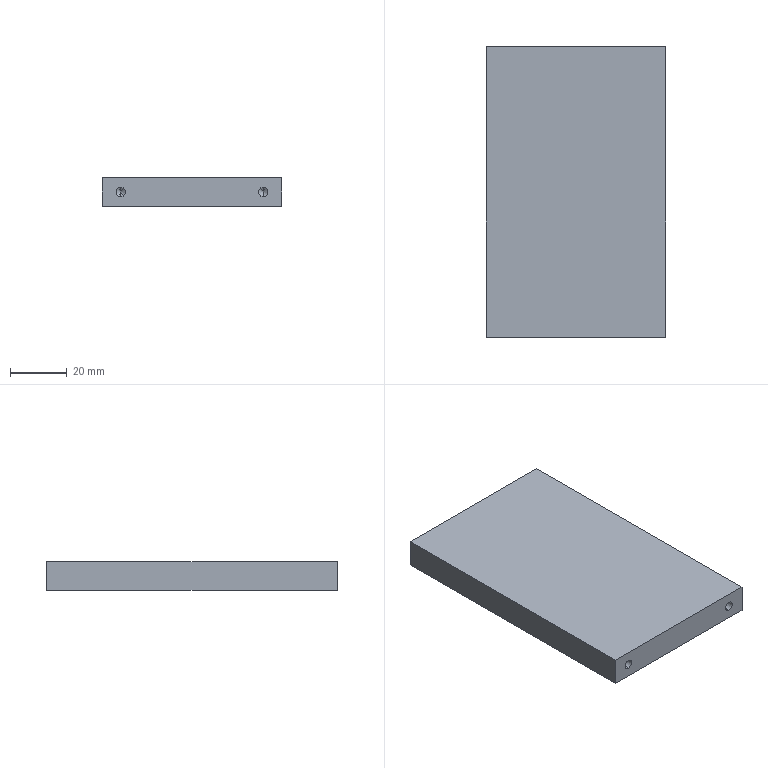Part | STEP file | 2033 Reinforcing rib | 1 solid | 22 faces | box 63 x 102 x 10 mm | volume 63855 mm3 | cylinder 8 | cone 8 | plane 6 | commonest cylinder face diameters 3.3 x8
STEP:
#1=CARTESIAN_POINT('',(0.,0.,0.));
#2=DIRECTION('',(0.,0.,1.));
#3=DIRECTION('',(1.,0.,0.));
#4=AXIS2_PLACEMENT_3D('',#1,#2,#3);
#5=CARTESIAN_POINT('',(56.5,90.5,6.65));
#6=VERTEX_POINT('',#5);
#7=CARTESIAN_POINT('',(56.5,102.,6.65));
#8=VERTEX_POINT('',#7);
#9=CARTESIAN_POINT('',(56.5,102.,6.65));
#10=DIRECTION('',(0.,1.,0.));
#11=VECTOR('',#10,1.);
#12=LINE('',#9,#11);
#13=CARTESIAN_POINT('',(56.5,102.,5.));
#14=DIRECTION('',(0.,1.,0.));
#15=DIRECTION('',(0.,0.,1.));
#16=AXIS2_PLACEMENT_3D('',#13,#14,#15);
#17=CYLINDRICAL_SURFACE('',#16,1.65);
#18=CARTESIAN_POINT('',(6.283,0.));
#19=DIRECTION('',(0.,1.));
#20=VECTOR('',#19,1.);
#21=LINE('',#18,#20);
#22=(GEOMETRIC_REPRESENTATION_CONTEXT(2)PARAMETRIC_REPRESENTATION_CONTEXT()REPRESENTATION_CONTEXT('',''));
#23=DEFINITIONAL_REPRESENTATION('',(#21),#22);
#24=PCURVE('',#17,#23);
#25=CARTESIAN_POINT('',(56.5,102.,5.));
#26=DIRECTION('',(0.,1.,0.));
#27=DIRECTION('',(0.,0.,1.));
#28=AXIS2_PLACEMENT_3D('',#25,#26,#27);
#29=CYLINDRICAL_SURFACE('',#28,1.65);
#30=CARTESIAN_POINT('',(0.,0.));
#31=DIRECTION('',(0.,1.));
#32=VECTOR('',#31,1.);
#33=LINE('',#30,#32);
#34=(GEOMETRIC_REPRESENTATION_CONTEXT(2)PARAMETRIC_REPRESENTATION_CONTEXT()REPRESENTATION_CONTEXT('',''));
#35=DEFINITIONAL_REPRESENTATION('',(#33),#34);
#36=PCURVE('',#29,#35);
#37=SURFACE_CURVE('',#12,(#24,#36),.PCURVE_S1.);
#38=EDGE_CURVE('',#6,#8,#37,.T.);
#39=ORIENTED_EDGE('',*,*,#38,.T.);
#40=CARTESIAN_POINT('',(56.5,102.,3.35));
#41=VERTEX_POINT('',#40);
#42=CARTESIAN_POINT('',(56.5,102.,5.));
#43=DIRECTION('',(0.,1.,0.));
#44=DIRECTION('',(0.,0.,1.));
#45=AXIS2_PLACEMENT_3D('',#42,#43,#44);
#46=CIRCLE('',#45,1.65);
#47=CARTESIAN_POINT('',(0.,0.));
#48=DIRECTION('',(1.,0.));
#49=VECTOR('',#48,1.);
#50=LINE('',#47,#49);
#51=(GEOMETRIC_REPRESENTATION_CONTEXT(2)PARAMETRIC_REPRESENTATION_CONTEXT()REPRESENTATION_CONTEXT('',''));
#52=DEFINITIONAL_REPRESENTATION('',(#50),#51);
#53=PCURVE('',#17,#52);
#54=CARTESIAN_POINT('',(63.,102.,10.));
#55=DIRECTION('',(0.,-1.,0.));
#56=DIRECTION('',(1.,0.,0.));
#57=AXIS2_PLACEMENT_3D('',#54,#55,#56);
#58=PLANE('',#57);
#59=CARTESIAN_POINT('',(-6.5,-3.35));
#60=CARTESIAN_POINT('',(-3.642,-3.35));
#61=CARTESIAN_POINT('',(-5.071,-5.825));
#62=CARTESIAN_POINT('',(-6.5,-8.3));
#63=CARTESIAN_POINT('',(-7.929,-5.825));
#64=CARTESIAN_POINT('',(-9.358,-3.35));
#65=CARTESIAN_POINT('',(-6.5,-3.35));
#66=(BOUNDED_CURVE()B_SPLINE_CURVE(2,(#59,#60,#61,#62,#63,#64,#65),.UNSPECIFIED.,.T.,.F.)B_SPLINE_CURVE_WITH_KNOTS((1,2,2,2,2,1),(-2.094,0.,2.094,4.189,6.283,8.378),.UNSPECIFIED.)CURVE()GEOMETRIC_REPRESENTATION_ITEM()RATIONAL_B_SPLINE_CURVE((1.,0.5,1.,0.5,1.,0.5,1.))REPRESENTATION_ITEM(''));
#67=(GEOMETRIC_REPRESENTATION_CONTEXT(2)PARAMETRIC_REPRESENTATION_CONTEXT()REPRESENTATION_CONTEXT('',''));
#68=DEFINITIONAL_REPRESENTATION('',(#66),#67);
#69=PCURVE('',#58,#68);
#70=SURFACE_CURVE('',#46,(#53,#69),.PCURVE_S1.);
#71=EDGE_CURVE('',#41,#8,#70,.T.);
#72=ORIENTED_EDGE('',*,*,#71,.F.);
#73=CARTESIAN_POINT('',(56.5,90.5,3.35));
#74=VERTEX_POINT('',#73);
#75=CARTESIAN_POINT('',(56.5,102.,3.35));
#76=DIRECTION('',(0.,1.,0.));
#77=VECTOR('',#76,1.);
#78=LINE('',#75,#77);
#79=CARTESIAN_POINT('',(3.142,0.));
#80=DIRECTION('',(0.,1.));
#81=VECTOR('',#80,1.);
#82=LINE('',#79,#81);
#83=(GEOMETRIC_REPRESENTATION_CONTEXT(2)PARAMETRIC_REPRESENTATION_CONTEXT()REPRESENTATION_CONTEXT('',''));
#84=DEFINITIONAL_REPRESENTATION('',(#82),#83);
#85=PCURVE('',#17,#84);
#86=CARTESIAN_POINT('',(3.142,0.));
#87=DIRECTION('',(0.,1.));
#88=VECTOR('',#87,1.);
#89=LINE('',#86,#88);
#90=(GEOMETRIC_REPRESENTATION_CONTEXT(2)PARAMETRIC_REPRESENTATION_CONTEXT()REPRESENTATION_CONTEXT('',''));
#91=DEFINITIONAL_REPRESENTATION('',(#89),#90);
#92=PCURVE('',#29,#91);
#93=SURFACE_CURVE('',#78,(#85,#92),.PCURVE_S1.);
#94=EDGE_CURVE('',#74,#41,#93,.T.);
#95=ORIENTED_EDGE('',*,*,#94,.F.);
#96=CARTESIAN_POINT('',(56.5,90.5,5.));
#97=DIRECTION('',(0.,1.,0.));
#98=DIRECTION('',(0.,0.,1.));
#99=AXIS2_PLACEMENT_3D('',#96,#97,#98);
#100=CIRCLE('',#99,1.65);
#101=CARTESIAN_POINT('',(0.,-11.5));
#102=DIRECTION('',(1.,0.));
#103=VECTOR('',#102,1.);
#104=LINE('',#101,#103);
#105=(GEOMETRIC_REPRESENTATION_CONTEXT(2)PARAMETRIC_REPRESENTATION_CONTEXT()REPRESENTATION_CONTEXT('',''));
#106=DEFINITIONAL_REPRESENTATION('',(#104),#105);
#107=PCURVE('',#17,#106);
#108=CARTESIAN_POINT('',(56.5,90.5,5.));
#109=DIRECTION('',(0.,1.,0.));
#110=DIRECTION('',(0.,0.,1.));
#111=AXIS2_PLACEMENT_3D('',#108,#109,#110);
#112=CONICAL_SURFACE('',#111,1.65,1.03);
#113=CARTESIAN_POINT('',(0.,0.));
#114=DIRECTION('',(1.,0.));
#115=VECTOR('',#114,1.);
#116=LINE('',#113,#115);
#117=(GEOMETRIC_REPRESENTATION_CONTEXT(2)PARAMETRIC_REPRESENTATION_CONTEXT()REPRESENTATION_CONTEXT('',''));
#118=DEFINITIONAL_REPRESENTATION('',(#116),#117);
#119=PCURVE('',#112,#118);
#120=SURFACE_CURVE('',#100,(#107,#119),.PCURVE_S1.);
#121=EDGE_CURVE('',#74,#6,#120,.T.);
#122=ORIENTED_EDGE('',*,*,#121,.T.);
#123=EDGE_LOOP('',(#39,#72,#95,#122));
#124=FACE_BOUND('',#123,.F.);
#125=ADVANCED_FACE('',(#124),#17,.F.);
#126=ORIENTED_EDGE('',*,*,#121,.F.);
#127=CARTESIAN_POINT('',(56.5,89.509,5.));
#128=VERTEX_POINT('',#127);
#129=CARTESIAN_POINT('',(56.5,90.5,3.35));
#130=DIRECTION('',(0.,0.515,-0.8572));
#131=VECTOR('',#130,1.);
#132=LINE('',#129,#131);
#133=CARTESIAN_POINT('',(3.142,0.));
#134=DIRECTION('',(0.,1.));
#135=VECTOR('',#134,1.);
#136=LINE('',#133,#135);
#137=(GEOMETRIC_REPRESENTATION_CONTEXT(2)PARAMETRIC_REPRESENTATION_CONTEXT()REPRESENTATION_CONTEXT('',''));
#138=DEFINITIONAL_REPRESENTATION('',(#136),#137);
#139=PCURVE('',#112,#138);
#140=CARTESIAN_POINT('',(56.5,90.5,5.));
#141=DIRECTION('',(0.,1.,0.));
#142=DIRECTION('',(0.,0.,1.));
#143=AXIS2_PLACEMENT_3D('',#140,#141,#142);
#144=CONICAL_SURFACE('',#143,1.65,1.03);
#145=CARTESIAN_POINT('',(3.142,0.));
#146=DIRECTION('',(0.,1.));
#147=VECTOR('',#146,1.);
#148=LINE('',#145,#147);
#149=(GEOMETRIC_REPRESENTATION_CONTEXT(2)PARAMETRIC_REPRESENTATION_CONTEXT()REPRESENTATION_CONTEXT('',''));
#150=DEFINITIONAL_REPRESENTATION('',(#148),#149);
#151=PCURVE('',#144,#150);
#152=SURFACE_CURVE('',#132,(#139,#151),.PCURVE_S1.);
#153=EDGE_CURVE('',#128,#74,#152,.T.);
#154=ORIENTED_EDGE('',*,*,#153,.F.);
#155=CARTESIAN_POINT('',(56.5,90.5,6.65));
#156=DIRECTION('',(0.,0.515,0.8572));
#157=VECTOR('',#156,1.);
#158=LINE('',#155,#157);
#159=CARTESIAN_POINT('',(6.283,0.));
#160=DIRECTION('',(0.,1.));
#161=VECTOR('',#160,1.);
#162=LINE('',#159,#161);
#163=(GEOMETRIC_REPRESENTATION_CONTEXT(2)PARAMETRIC_REPRESENTATION_CONTEXT()REPRESENTATION_CONTEXT('',''));
#164=DEFINITIONAL_REPRESENTATION('',(#162),#163);
#165=PCURVE('',#112,#164);
#166=CARTESIAN_POINT('',(0.,0.));
#167=DIRECTION('',(0.,1.));
#168=VECTOR('',#167,1.);
#169=LINE('',#166,#168);
#170=(GEOMETRIC_REPRESENTATION_CONTEXT(2)PARAMETRIC_REPRESENTATION_CONTEXT()REPRESENTATION_CONTEXT('',''));
#171=DEFINITIONAL_REPRESENTATION('',(#169),#170);
#172=PCURVE('',#144,#171);
#173=SURFACE_CURVE('',#158,(#165,#172),.PCURVE_S1.);
#174=EDGE_CURVE('',#128,#6,#173,.T.);
#175=ORIENTED_EDGE('',*,*,#174,.T.);
#176=EDGE_LOOP('',(#126,#154,#175));
#177=FACE_BOUND('',#176,.F.);
#178=ADVANCED_FACE('',(#177),#112,.F.);
#179=CARTESIAN_POINT('',(6.5,90.5,6.65));
#180=VERTEX_POINT('',#179);
#181=CARTESIAN_POINT('',(6.5,102.,6.65));
#182=VERTEX_POINT('',#181);
#183=CARTESIAN_POINT('',(6.5,102.,6.65));
#184=DIRECTION('',(0.,1.,0.));
#185=VECTOR('',#184,1.);
#186=LINE('',#183,#185);
#187=CARTESIAN_POINT('',(6.5,102.,5.));
#188=DIRECTION('',(0.,1.,0.));
#189=DIRECTION('',(0.,0.,1.));
#190=AXIS2_PLACEMENT_3D('',#187,#188,#189);
#191=CYLINDRICAL_SURFACE('',#190,1.65);
#192=CARTESIAN_POINT('',(6.283,0.));
#193=DIRECTION('',(0.,1.));
#194=VECTOR('',#193,1.);
#195=LINE('',#192,#194);
#196=(GEOMETRIC_REPRESENTATION_CONTEXT(2)PARAMETRIC_REPRESENTATION_CONTEXT()REPRESENTATION_CONTEXT('',''));
#197=DEFINITIONAL_REPRESENTATION('',(#195),#196);
#198=PCURVE('',#191,#197);
#199=CARTESIAN_POINT('',(6.5,102.,5.));
#200=DIRECTION('',(0.,1.,0.));
#201=DIRECTION('',(0.,0.,1.));
#202=AXIS2_PLACEMENT_3D('',#199,#200,#201);
#203=CYLINDRICAL_SURFACE('',#202,1.65);
#204=CARTESIAN_POINT('',(0.,0.));
#205=DIRECTION('',(0.,1.));
#206=VECTOR('',#205,1.);
#207=LINE('',#204,#206);
#208=(GEOMETRIC_REPRESENTATION_CONTEXT(2)PARAMETRIC_REPRESENTATION_CONTEXT()REPRESENTATION_CONTEXT('',''));
#209=DEFINITIONAL_REPRESENTATION('',(#207),#208);
#210=PCURVE('',#203,#209);
#211=SURFACE_CURVE('',#186,(#198,#210),.PCURVE_S1.);
#212=EDGE_CURVE('',#180,#182,#211,.T.);
#213=ORIENTED_EDGE('',*,*,#212,.T.);
#214=CARTESIAN_POINT('',(6.5,102.,3.35));
#215=VERTEX_POINT('',#214);
#216=CARTESIAN_POINT('',(6.5,102.,5.));
#217=DIRECTION('',(0.,1.,0.));
#218=DIRECTION('',(0.,0.,1.));
#219=AXIS2_PLACEMENT_3D('',#216,#217,#218);
#220=CIRCLE('',#219,1.65);
#221=CARTESIAN_POINT('',(0.,0.));
#222=DIRECTION('',(1.,0.));
#223=VECTOR('',#222,1.);
#224=LINE('',#221,#223);
#225=(GEOMETRIC_REPRESENTATION_CONTEXT(2)PARAMETRIC_REPRESENTATION_CONTEXT()REPRESENTATION_CONTEXT('',''));
#226=DEFINITIONAL_REPRESENTATION('',(#224),#225);
#227=PCURVE('',#191,#226);
#228=CARTESIAN_POINT('',(-56.5,-3.35));
#229=CARTESIAN_POINT('',(-53.642,-3.35));
#230=CARTESIAN_POINT('',(-55.071,-5.825));
#231=CARTESIAN_POINT('',(-56.5,-8.3));
#232=CARTESIAN_POINT('',(-57.929,-5.825));
#233=CARTESIAN_POINT('',(-59.358,-3.35));
#234=CARTESIAN_POINT('',(-56.5,-3.35));
#235=(BOUNDED_CURVE()B_SPLINE_CURVE(2,(#228,#229,#230,#231,#232,#233,#234),.UNSPECIFIED.,.T.,.F.)B_SPLINE_CURVE_WITH_KNOTS((1,2,2,2,2,1),(-2.094,0.,2.094,4.189,6.283,8.378),.UNSPECIFIED.)CURVE()GEOMETRIC_REPRESENTATION_ITEM()RATIONAL_B_SPLINE_CURVE((1.,0.5,1.,0.5,1.,0.5,1.))REPRESENTATION_ITEM(''));
#236=(GEOMETRIC_REPRESENTATION_CONTEXT(2)PARAMETRIC_REPRESENTATION_CONTEXT()REPRESENTATION_CONTEXT('',''));
#237=DEFINITIONAL_REPRESENTATION('',(#235),#236);
#238=PCURVE('',#58,#237);
#239=SURFACE_CURVE('',#220,(#227,#238),.PCURVE_S1.);
#240=EDGE_CURVE('',#215,#182,#239,.T.);
#241=ORIENTED_EDGE('',*,*,#240,.F.);
#242=CARTESIAN_POINT('',(6.5,90.5,3.35));
#243=VERTEX_POINT('',#242);
#244=CARTESIAN_POINT('',(6.5,102.,3.35));
#245=DIRECTION('',(0.,1.,0.));
#246=VECTOR('',#245,1.);
#247=LINE('',#244,#246);
#248=CARTESIAN_POINT('',(3.142,0.));
#249=DIRECTION('',(0.,1.));
#250=VECTOR('',#249,1.);
#251=LINE('',#248,#250);
#252=(GEOMETRIC_REPRESENTATION_CONTEXT(2)PARAMETRIC_REPRESENTATION_CONTEXT()REPRESENTATION_CONTEXT('',''));
#253=DEFINITIONAL_REPRESENTATION('',(#251),#252);
#254=PCURVE('',#191,#253);
#255=CARTESIAN_POINT('',(3.142,0.));
#256=DIRECTION('',(0.,1.));
#257=VECTOR('',#256,1.);
#258=LINE('',#255,#257);
#259=(GEOMETRIC_REPRESENTATION_CONTEXT(2)PARAMETRIC_REPRESENTATION_CONTEXT()REPRESENTATION_CONTEXT('',''));
#260=DEFINITIONAL_REPRESENTATION('',(#258),#259);
#261=PCURVE('',#203,#260);
#262=SURFACE_CURVE('',#247,(#254,#261),.PCURVE_S1.);
#263=EDGE_CURVE('',#243,#215,#262,.T.);
#264=ORIENTED_EDGE('',*,*,#263,.F.);
#265=CARTESIAN_POINT('',(6.5,90.5,5.));
#266=DIRECTION('',(0.,1.,0.));
#267=DIRECTION('',(0.,0.,1.));
#268=AXIS2_PLACEMENT_3D('',#265,#266,#267);
#269=CIRCLE('',#268,1.65);
#270=CARTESIAN_POINT('',(0.,-11.5));
#271=DIRECTION('',(1.,0.));
#272=VECTOR('',#271,1.);
#273=LINE('',#270,#272);
#274=(GEOMETRIC_REPRESENTATION_CONTEXT(2)PARAMETRIC_REPRESENTATION_CONTEXT()REPRESENTATION_CONTEXT('',''));
#275=DEFINITIONAL_REPRESENTATION('',(#273),#274);
#276=PCURVE('',#191,#275);
#277=CARTESIAN_POINT('',(6.5,90.5,5.));
#278=DIRECTION('',(0.,1.,0.));
#279=DIRECTION('',(0.,0.,1.));
#280=AXIS2_PLACEMENT_3D('',#277,#278,#279);
#281=CONICAL_SURFACE('',#280,1.65,1.03);
#282=CARTESIAN_POINT('',(0.,0.));
#283=DIRECTION('',(1.,0.));
#284=VECTOR('',#283,1.);
#285=LINE('',#282,#284);
#286=(GEOMETRIC_REPRESENTATION_CONTEXT(2)PARAMETRIC_REPRESENTATION_CONTEXT()REPRESENTATION_CONTEXT('',''));
#287=DEFINITIONAL_REPRESENTATION('',(#285),#286);
#288=PCURVE('',#281,#287);
#289=SURFACE_CURVE('',#269,(#276,#288),.PCURVE_S1.);
#290=EDGE_CURVE('',#243,#180,#289,.T.);
#291=ORIENTED_EDGE('',*,*,#290,.T.);
#292=EDGE_LOOP('',(#213,#241,#264,#291));
#293=FACE_BOUND('',#292,.F.);
#294=ADVANCED_FACE('',(#293),#191,.F.);
#295=ORIENTED_EDGE('',*,*,#290,.F.);
#296=CARTESIAN_POINT('',(6.5,89.509,5.));
#297=VERTEX_POINT('',#296);
#298=CARTESIAN_POINT('',(6.5,90.5,3.35));
#299=DIRECTION('',(0.,0.515,-0.8572));
#300=VECTOR('',#299,1.);
#301=LINE('',#298,#300);
#302=CARTESIAN_POINT('',(3.142,0.));
#303=DIRECTION('',(0.,1.));
#304=VECTOR('',#303,1.);
#305=LINE('',#302,#304);
#306=(GEOMETRIC_REPRESENTATION_CONTEXT(2)PARAMETRIC_REPRESENTATION_CONTEXT()REPRESENTATION_CONTEXT('',''));
#307=DEFINITIONAL_REPRESENTATION('',(#305),#306);
#308=PCURVE('',#281,#307);
#309=CARTESIAN_POINT('',(6.5,90.5,5.));
#310=DIRECTION('',(0.,1.,0.));
#311=DIRECTION('',(0.,0.,1.));
#312=AXIS2_PLACEMENT_3D('',#309,#310,#311);
#313=CONICAL_SURFACE('',#312,1.65,1.03);
#314=CARTESIAN_POINT('',(3.142,0.));
#315=DIRECTION('',(0.,1.));
#316=VECTOR('',#315,1.);
#317=LINE('',#314,#316);
#318=(GEOMETRIC_REPRESENTATION_CONTEXT(2)PARAMETRIC_REPRESENTATION_CONTEXT()REPRESENTATION_CONTEXT('',''));
#319=DEFINITIONAL_REPRESENTATION('',(#317),#318);
#320=PCURVE('',#313,#319);
#321=SURFACE_CURVE('',#301,(#308,#320),.PCURVE_S1.);
#322=EDGE_CURVE('',#297,#243,#321,.T.);
#323=ORIENTED_EDGE('',*,*,#322,.F.);
#324=CARTESIAN_POINT('',(6.5,90.5,6.65));
#325=DIRECTION('',(0.,0.515,0.8572));
#326=VECTOR('',#325,1.);
#327=LINE('',#324,#326);
#328=CARTESIAN_POINT('',(6.283,0.));
#329=DIRECTION('',(0.,1.));
#330=VECTOR('',#329,1.);
#331=LINE('',#328,#330);
#332=(GEOMETRIC_REPRESENTATION_CONTEXT(2)PARAMETRIC_REPRESENTATION_CONTEXT()REPRESENTATION_CONTEXT('',''));
#333=DEFINITIONAL_REPRESENTATION('',(#331),#332);
#334=PCURVE('',#281,#333);
#335=CARTESIAN_POINT('',(0.,0.));
#336=DIRECTION('',(0.,1.));
#337=VECTOR('',#336,1.);
#338=LINE('',#335,#337);
#339=(GEOMETRIC_REPRESENTATION_CONTEXT(2)PARAMETRIC_REPRESENTATION_CONTEXT()REPRESENTATION_CONTEXT('',''));
#340=DEFINITIONAL_REPRESENTATION('',(#338),#339);
#341=PCURVE('',#313,#340);
#342=SURFACE_CURVE('',#327,(#334,#341),.PCURVE_S1.);
#343=EDGE_CURVE('',#297,#180,#342,.T.);
#344=ORIENTED_EDGE('',*,*,#343,.T.);
#345=EDGE_LOOP('',(#295,#323,#344));
#346=FACE_BOUND('',#345,.F.);
#347=ADVANCED_FACE('',(#346),#281,.F.);
#348=CARTESIAN_POINT('',(6.5,11.5,3.35));
#349=VERTEX_POINT('',#348);
#350=CARTESIAN_POINT('',(6.5,0.,3.35));
#351=VERTEX_POINT('',#350);
#352=CARTESIAN_POINT('',(6.5,0.,3.35));
#353=DIRECTION('',(0.,-1.,0.));
#354=VECTOR('',#353,1.);
#355=LINE('',#352,#354);
#356=CARTESIAN_POINT('',(6.5,0.,5.));
#357=DIRECTION('',(0.,-1.,0.));
#358=DIRECTION('',(0.,0.,-1.));
#359=AXIS2_PLACEMENT_3D('',#356,#357,#358);
#360=CYLINDRICAL_SURFACE('',#359,1.65);
#361=CARTESIAN_POINT('',(6.283,0.));
#362=DIRECTION('',(0.,1.));
#363=VECTOR('',#362,1.);
#364=LINE('',#361,#363);
#365=(GEOMETRIC_REPRESENTATION_CONTEXT(2)PARAMETRIC_REPRESENTATION_CONTEXT()REPRESENTATION_CONTEXT('',''));
#366=DEFINITIONAL_REPRESENTATION('',(#364),#365);
#367=PCURVE('',#360,#366);
#368=CARTESIAN_POINT('',(6.5,0.,5.));
#369=DIRECTION('',(0.,-1.,0.));
#370=DIRECTION('',(0.,0.,-1.));
#371=AXIS2_PLACEMENT_3D('',#368,#369,#370);
#372=CYLINDRICAL_SURFACE('',#371,1.65);
#373=CARTESIAN_POINT('',(0.,0.));
#374=DIRECTION('',(0.,1.));
#375=VECTOR('',#374,1.);
#376=LINE('',#373,#375);
#377=(GEOMETRIC_REPRESENTATION_CONTEXT(2)PARAMETRIC_REPRESENTATION_CONTEXT()REPRESENTATION_CONTEXT('',''));
#378=DEFINITIONAL_REPRESENTATION('',(#376),#377);
#379=PCURVE('',#372,#378);
#380=SURFACE_CURVE('',#355,(#367,#379),.PCURVE_S1.);
#381=EDGE_CURVE('',#349,#351,#380,.T.);
#382=ORIENTED_EDGE('',*,*,#381,.T.);
#383=CARTESIAN_POINT('',(6.5,0.,6.65));
#384=VERTEX_POINT('',#383);
#385=CARTESIAN_POINT('',(6.5,0.,5.));
#386=DIRECTION('',(0.,-1.,0.));
#387=DIRECTION('',(0.,0.,-1.));
#388=AXIS2_PLACEMENT_3D('',#385,#386,#387);
#389=CIRCLE('',#388,1.65);
#390=CARTESIAN_POINT('',(0.,0.));
#391=DIRECTION('',(1.,0.));
#392=VECTOR('',#391,1.);
#393=LINE('',#390,#392);
#394=(GEOMETRIC_REPRESENTATION_CONTEXT(2)PARAMETRIC_REPRESENTATION_CONTEXT()REPRESENTATION_CONTEXT('',''));
#395=DEFINITIONAL_REPRESENTATION('',(#393),#394);
#396=PCURVE('',#360,#395);
#397=CARTESIAN_POINT('',(0.,0.,10.));
#398=DIRECTION('',(0.,1.,0.));
#399=DIRECTION('',(0.,0.,1.));
#400=AXIS2_PLACEMENT_3D('',#397,#398,#399);
#401=PLANE('',#400);
#402=CARTESIAN_POINT('',(-6.65,6.5));
#403=CARTESIAN_POINT('',(-6.65,9.358));
#404=CARTESIAN_POINT('',(-4.175,7.929));
#405=CARTESIAN_POINT('',(-1.7,6.5));
#406=CARTESIAN_POINT('',(-4.175,5.071));
#407=CARTESIAN_POINT('',(-6.65,3.642));
#408=CARTESIAN_POINT('',(-6.65,6.5));
#409=(BOUNDED_CURVE()B_SPLINE_CURVE(2,(#402,#403,#404,#405,#406,#407,#408),.UNSPECIFIED.,.T.,.F.)B_SPLINE_CURVE_WITH_KNOTS((1,2,2,2,2,1),(-2.094,0.,2.094,4.189,6.283,8.378),.UNSPECIFIED.)CURVE()GEOMETRIC_REPRESENTATION_ITEM()RATIONAL_B_SPLINE_CURVE((1.,0.5,1.,0.5,1.,0.5,1.))REPRESENTATION_ITEM(''));
#410=(GEOMETRIC_REPRESENTATION_CONTEXT(2)PARAMETRIC_REPRESENTATION_CONTEXT()REPRESENTATION_CONTEXT('',''));
#411=DEFINITIONAL_REPRESENTATION('',(#409),#410);
#412=PCURVE('',#401,#411);
#413=SURFACE_CURVE('',#389,(#396,#412),.PCURVE_S1.);
#414=EDGE_CURVE('',#384,#351,#413,.T.);
#415=ORIENTED_EDGE('',*,*,#414,.F.);
#416=CARTESIAN_POINT('',(6.5,11.5,6.65));
#417=VERTEX_POINT('',#416);
#418=CARTESIAN_POINT('',(6.5,0.,6.65));
#419=DIRECTION('',(0.,-1.,0.));
#420=VECTOR('',#419,1.);
#421=LINE('',#418,#420);
#422=CARTESIAN_POINT('',(3.142,0.));
#423=DIRECTION('',(0.,1.));
#424=VECTOR('',#423,1.);
#425=LINE('',#422,#424);
#426=(GEOMETRIC_REPRESENTATION_CONTEXT(2)PARAMETRIC_REPRESENTATION_CONTEXT()REPRESENTATION_CONTEXT('',''));
#427=DEFINITIONAL_REPRESENTATION('',(#425),#426);
#428=PCURVE('',#360,#427);
#429=CARTESIAN_POINT('',(3.142,0.));
#430=DIRECTION('',(0.,1.));
#431=VECTOR('',#430,1.);
#432=LINE('',#429,#431);
#433=(GEOMETRIC_REPRESENTATION_CONTEXT(2)PARAMETRIC_REPRESENTATION_CONTEXT()REPRESENTATION_CONTEXT('',''));
#434=DEFINITIONAL_REPRESENTATION('',(#432),#433);
#435=PCURVE('',#372,#434);
#436=SURFACE_CURVE('',#421,(#428,#435),.PCURVE_S1.);
#437=EDGE_CURVE('',#417,#384,#436,.T.);
#438=ORIENTED_EDGE('',*,*,#437,.F.);
#439=CARTESIAN_POINT('',(6.5,11.5,5.));
#440=DIRECTION('',(0.,-1.,0.));
#441=DIRECTION('',(0.,0.,-1.));
#442=AXIS2_PLACEMENT_3D('',#439,#440,#441);
#443=CIRCLE('',#442,1.65);
#444=CARTESIAN_POINT('',(0.,-11.5));
#445=DIRECTION('',(1.,0.));
#446=VECTOR('',#445,1.);
#447=LINE('',#444,#446);
#448=(GEOMETRIC_REPRESENTATION_CONTEXT(2)PARAMETRIC_REPRESENTATION_CONTEXT()REPRESENTATION_CONTEXT('',''));
#449=DEFINITIONAL_REPRESENTATION('',(#447),#448);
#450=PCURVE('',#360,#449);
#451=CARTESIAN_POINT('',(6.5,11.5,5.));
#452=DIRECTION('',(0.,-1.,0.));
#453=DIRECTION('',(0.,0.,-1.));
#454=AXIS2_PLACEMENT_3D('',#451,#452,#453);
#455=CONICAL_SURFACE('',#454,1.65,1.03);
#456=CARTESIAN_POINT('',(0.,0.));
#457=DIRECTION('',(1.,0.));
#458=VECTOR('',#457,1.);
#459=LINE('',#456,#458);
#460=(GEOMETRIC_REPRESENTATION_CONTEXT(2)PARAMETRIC_REPRESENTATION_CONTEXT()REPRESENTATION_CONTEXT('',''));
#461=DEFINITIONAL_REPRESENTATION('',(#459),#460);
#462=PCURVE('',#455,#461);
#463=SURFACE_CURVE('',#443,(#450,#462),.PCURVE_S1.);
#464=EDGE_CURVE('',#417,#349,#463,.T.);
#465=ORIENTED_EDGE('',*,*,#464,.T.);
#466=EDGE_LOOP('',(#382,#415,#438,#465));
#467=FACE_BOUND('',#466,.F.);
#468=ADVANCED_FACE('',(#467),#360,.F.);
#469=ORIENTED_EDGE('',*,*,#464,.F.);
#470=CARTESIAN_POINT('',(6.5,12.491,5.));
#471=VERTEX_POINT('',#470);
#472=CARTESIAN_POINT('',(6.5,11.5,6.65));
#473=DIRECTION('',(0.,-0.515,0.8572));
#474=VECTOR('',#473,1.);
#475=LINE('',#472,#474);
#476=CARTESIAN_POINT('',(3.142,0.));
#477=DIRECTION('',(0.,1.));
#478=VECTOR('',#477,1.);
#479=LINE('',#476,#478);
#480=(GEOMETRIC_REPRESENTATION_CONTEXT(2)PARAMETRIC_REPRESENTATION_CONTEXT()REPRESENTATION_CONTEXT('',''));
#481=DEFINITIONAL_REPRESENTATION('',(#479),#480);
#482=PCURVE('',#455,#481);
#483=CARTESIAN_POINT('',(6.5,11.5,5.));
#484=DIRECTION('',(0.,-1.,0.));
#485=DIRECTION('',(0.,0.,-1.));
#486=AXIS2_PLACEMENT_3D('',#483,#484,#485);
#487=CONICAL_SURFACE('',#486,1.65,1.03);
#488=CARTESIAN_POINT('',(3.142,0.));
#489=DIRECTION('',(0.,1.));
#490=VECTOR('',#489,1.);
#491=LINE('',#488,#490);
#492=(GEOMETRIC_REPRESENTATION_CONTEXT(2)PARAMETRIC_REPRESENTATION_CONTEXT()REPRESENTATION_CONTEXT('',''));
#493=DEFINITIONAL_REPRESENTATION('',(#491),#492);
#494=PCURVE('',#487,#493);
#495=SURFACE_CURVE('',#475,(#482,#494),.PCURVE_S1.);
#496=EDGE_CURVE('',#471,#417,#495,.T.);
#497=ORIENTED_EDGE('',*,*,#496,.F.);
#498=CARTESIAN_POINT('',(6.5,11.5,3.35));
#499=DIRECTION('',(0.,-0.515,-0.8572));
#500=VECTOR('',#499,1.);
#501=LINE('',#498,#500);
#502=CARTESIAN_POINT('',(6.283,0.));
#503=DIRECTION('',(0.,1.));
#504=VECTOR('',#503,1.);
#505=LINE('',#502,#504);
#506=(GEOMETRIC_REPRESENTATION_CONTEXT(2)PARAMETRIC_REPRESENTATION_CONTEXT()REPRESENTATION_CONTEXT('',''));
#507=DEFINITIONAL_REPRESENTATION('',(#505),#506);
#508=PCURVE('',#455,#507);
#509=CARTESIAN_POINT('',(0.,0.));
#510=DIRECTION('',(0.,1.));
#511=VECTOR('',#510,1.);
#512=LINE('',#509,#511);
#513=(GEOMETRIC_REPRESENTATION_CONTEXT(2)PARAMETRIC_REPRESENTATION_CONTEXT()REPRESENTATION_CONTEXT('',''));
#514=DEFINITIONAL_REPRESENTATION('',(#512),#513);
#515=PCURVE('',#487,#514);
#516=SURFACE_CURVE('',#501,(#508,#515),.PCURVE_S1.);
#517=EDGE_CURVE('',#471,#349,#516,.T.);
#518=ORIENTED_EDGE('',*,*,#517,.T.);
#519=EDGE_LOOP('',(#469,#497,#518));
#520=FACE_BOUND('',#519,.F.);
#521=ADVANCED_FACE('',(#520),#455,.F.);
#522=CARTESIAN_POINT('',(56.5,11.5,3.35));
#523=VERTEX_POINT('',#522);
#524=CARTESIAN_POINT('',(56.5,0.,3.35));
#525=VERTEX_POINT('',#524);
#526=CARTESIAN_POINT('',(56.5,0.,3.35));
#527=DIRECTION('',(0.,-1.,0.));
#528=VECTOR('',#527,1.);
#529=LINE('',#526,#528);
#530=CARTESIAN_POINT('',(56.5,0.,5.));
#531=DIRECTION('',(0.,-1.,0.));
#532=DIRECTION('',(0.,0.,-1.));
#533=AXIS2_PLACEMENT_3D('',#530,#531,#532);
#534=CYLINDRICAL_SURFACE('',#533,1.65);
#535=CARTESIAN_POINT('',(6.283,0.));
#536=DIRECTION('',(0.,1.));
#537=VECTOR('',#536,1.);
#538=LINE('',#535,#537);
#539=(GEOMETRIC_REPRESENTATION_CONTEXT(2)PARAMETRIC_REPRESENTATION_CONTEXT()REPRESENTATION_CONTEXT('',''));
#540=DEFINITIONAL_REPRESENTATION('',(#538),#539);
#541=PCURVE('',#534,#540);
#542=CARTESIAN_POINT('',(56.5,0.,5.));
#543=DIRECTION('',(0.,-1.,0.));
#544=DIRECTION('',(0.,0.,-1.));
#545=AXIS2_PLACEMENT_3D('',#542,#543,#544);
#546=CYLINDRICAL_SURFACE('',#545,1.65);
#547=CARTESIAN_POINT('',(0.,0.));
#548=DIRECTION('',(0.,1.));
#549=VECTOR('',#548,1.);
#550=LINE('',#547,#549);
#551=(GEOMETRIC_REPRESENTATION_CONTEXT(2)PARAMETRIC_REPRESENTATION_CONTEXT()REPRESENTATION_CONTEXT('',''));
#552=DEFINITIONAL_REPRESENTATION('',(#550),#551);
#553=PCURVE('',#546,#552);
#554=SURFACE_CURVE('',#529,(#541,#553),.PCURVE_S1.);
#555=EDGE_CURVE('',#523,#525,#554,.T.);
#556=ORIENTED_EDGE('',*,*,#555,.T.);
#557=CARTESIAN_POINT('',(56.5,0.,6.65));
#558=VERTEX_POINT('',#557);
#559=CARTESIAN_POINT('',(56.5,0.,5.));
#560=DIRECTION('',(0.,-1.,0.));
#561=DIRECTION('',(0.,0.,-1.));
#562=AXIS2_PLACEMENT_3D('',#559,#560,#561);
#563=CIRCLE('',#562,1.65);
#564=CARTESIAN_POINT('',(0.,0.));
#565=DIRECTION('',(1.,0.));
#566=VECTOR('',#565,1.);
#567=LINE('',#564,#566);
#568=(GEOMETRIC_REPRESENTATION_CONTEXT(2)PARAMETRIC_REPRESENTATION_CONTEXT()REPRESENTATION_CONTEXT('',''));
#569=DEFINITIONAL_REPRESENTATION('',(#567),#568);
#570=PCURVE('',#534,#569);
#571=CARTESIAN_POINT('',(-6.65,56.5));
#572=CARTESIAN_POINT('',(-6.65,59.358));
#573=CARTESIAN_POINT('',(-4.175,57.929));
#574=CARTESIAN_POINT('',(-1.7,56.5));
#575=CARTESIAN_POINT('',(-4.175,55.071));
#576=CARTESIAN_POINT('',(-6.65,53.642));
#577=CARTESIAN_POINT('',(-6.65,56.5));
#578=(BOUNDED_CURVE()B_SPLINE_CURVE(2,(#571,#572,#573,#574,#575,#576,#577),.UNSPECIFIED.,.T.,.F.)B_SPLINE_CURVE_WITH_KNOTS((1,2,2,2,2,1),(-2.094,0.,2.094,4.189,6.283,8.378),.UNSPECIFIED.)CURVE()GEOMETRIC_REPRESENTATION_ITEM()RATIONAL_B_SPLINE_CURVE((1.,0.5,1.,0.5,1.,0.5,1.))REPRESENTATION_ITEM(''));
#579=(GEOMETRIC_REPRESENTATION_CONTEXT(2)PARAMETRIC_REPRESENTATION_CONTEXT()REPRESENTATION_CONTEXT('',''));
#580=DEFINITIONAL_REPRESENTATION('',(#578),#579);
#581=PCURVE('',#401,#580);
#582=SURFACE_CURVE('',#563,(#570,#581),.PCURVE_S1.);
#583=EDGE_CURVE('',#558,#525,#582,.T.);
#584=ORIENTED_EDGE('',*,*,#583,.F.);
#585=CARTESIAN_POINT('',(56.5,11.5,6.65));
#586=VERTEX_POINT('',#585);
#587=CARTESIAN_POINT('',(56.5,0.,6.65));
#588=DIRECTION('',(0.,-1.,0.));
#589=VECTOR('',#588,1.);
#590=LINE('',#587,#589);
#591=CARTESIAN_POINT('',(3.142,0.));
#592=DIRECTION('',(0.,1.));
#593=VECTOR('',#592,1.);
#594=LINE('',#591,#593);
#595=(GEOMETRIC_REPRESENTATION_CONTEXT(2)PARAMETRIC_REPRESENTATION_CONTEXT()REPRESENTATION_CONTEXT('',''));
#596=DEFINITIONAL_REPRESENTATION('',(#594),#595);
#597=PCURVE('',#534,#596);
#598=CARTESIAN_POINT('',(3.142,0.));
#599=DIRECTION('',(0.,1.));
#600=VECTOR('',#599,1.);
#601=LINE('',#598,#600);
#602=(GEOMETRIC_REPRESENTATION_CONTEXT(2)PARAMETRIC_REPRESENTATION_CONTEXT()REPRESENTATION_CONTEXT('',''));
#603=DEFINITIONAL_REPRESENTATION('',(#601),#602);
#604=PCURVE('',#546,#603);
#605=SURFACE_CURVE('',#590,(#597,#604),.PCURVE_S1.);
#606=EDGE_CURVE('',#586,#558,#605,.T.);
#607=ORIENTED_EDGE('',*,*,#606,.F.);
#608=CARTESIAN_POINT('',(56.5,11.5,5.));
#609=DIRECTION('',(0.,-1.,0.));
#610=DIRECTION('',(0.,0.,-1.));
#611=AXIS2_PLACEMENT_3D('',#608,#609,#610);
#612=CIRCLE('',#611,1.65);
#613=CARTESIAN_POINT('',(0.,-11.5));
#614=DIRECTION('',(1.,0.));
#615=VECTOR('',#614,1.);
#616=LINE('',#613,#615);
#617=(GEOMETRIC_REPRESENTATION_CONTEXT(2)PARAMETRIC_REPRESENTATION_CONTEXT()REPRESENTATION_CONTEXT('',''));
#618=DEFINITIONAL_REPRESENTATION('',(#616),#617);
#619=PCURVE('',#534,#618);
#620=CARTESIAN_POINT('',(56.5,11.5,5.));
#621=DIRECTION('',(0.,-1.,0.));
#622=DIRECTION('',(0.,0.,-1.));
#623=AXIS2_PLACEMENT_3D('',#620,#621,#622);
#624=CONICAL_SURFACE('',#623,1.65,1.03);
#625=CARTESIAN_POINT('',(0.,0.));
#626=DIRECTION('',(1.,0.));
#627=VECTOR('',#626,1.);
#628=LINE('',#625,#627);
#629=(GEOMETRIC_REPRESENTATION_CONTEXT(2)PARAMETRIC_REPRESENTATION_CONTEXT()REPRESENTATION_CONTEXT('',''));
#630=DEFINITIONAL_REPRESENTATION('',(#628),#629);
#631=PCURVE('',#624,#630);
#632=SURFACE_CURVE('',#612,(#619,#631),.PCURVE_S1.);
#633=EDGE_CURVE('',#586,#523,#632,.T.);
#634=ORIENTED_EDGE('',*,*,#633,.T.);
#635=EDGE_LOOP('',(#556,#584,#607,#634));
#636=FACE_BOUND('',#635,.F.);
#637=ADVANCED_FACE('',(#636),#534,.F.);
#638=ORIENTED_EDGE('',*,*,#633,.F.);
#639=CARTESIAN_POINT('',(56.5,12.491,5.));
#640=VERTEX_POINT('',#639);
#641=CARTESIAN_POINT('',(56.5,11.5,6.65));
#642=DIRECTION('',(0.,-0.515,0.8572));
#643=VECTOR('',#642,1.);
#644=LINE('',#641,#643);
#645=CARTESIAN_POINT('',(3.142,-0.9914));
#646=CARTESIAN_POINT('',(3.142,-0.9764));
#647=CARTESIAN_POINT('',(3.142,-0.9464));
#648=CARTESIAN_POINT('',(3.142,-0.9013));
#649=CARTESIAN_POINT('',(3.142,-0.8562));
#650=CARTESIAN_POINT('',(3.142,-0.8112));
#651=CARTESIAN_POINT('',(3.142,-0.7661));
#652=CARTESIAN_POINT('',(3.142,-0.721));
#653=CARTESIAN_POINT('',(3.142,-0.676));
#654=CARTESIAN_POINT('',(3.142,-0.6309));
#655=CARTESIAN_POINT('',(3.142,-0.5858));
#656=CARTESIAN_POINT('',(3.142,-0.5408));
#657=CARTESIAN_POINT('',(3.142,-0.4957));
#658=CARTESIAN_POINT('',(3.142,-0.4506));
#659=CARTESIAN_POINT('',(3.142,-0.4056));
#660=CARTESIAN_POINT('',(3.142,-0.3605));
#661=CARTESIAN_POINT('',(3.142,-0.3155));
#662=CARTESIAN_POINT('',(3.142,-0.2704));
#663=CARTESIAN_POINT('',(3.142,-0.2253));
#664=CARTESIAN_POINT('',(3.142,-0.1803));
#665=CARTESIAN_POINT('',(3.142,-0.1352));
#666=CARTESIAN_POINT('',(3.142,-0.09013));
#667=CARTESIAN_POINT('',(3.142,-0.04506));
#668=CARTESIAN_POINT('',(3.142,-0.01502));
#669=CARTESIAN_POINT('',(3.142,0.));
#670=B_SPLINE_CURVE_WITH_KNOTS('',3,(#645,#646,#647,#648,#649,#650,#651,#652,#653,#654,#655,#656,#657,#658,#659,#660,#661,#662,#663,#664,#665,#666,#667,#668,#669),.UNSPECIFIED.,.F.,.F.,(4,1,1,1,1,1,1,1,1,1,1,1,1,1,1,1,1,1,1,1,1,1,4),(-1.925,-1.837,-1.75,-1.662,-1.575,-1.487,-1.4,-1.312,-1.225,-1.137,-1.05,-0.9625,-0.875,-0.7875,-0.7,-0.6125,-0.525,-0.4375,-0.35,-0.2625,-0.175,-0.0875,0.),.QUASI_UNIFORM_KNOTS.);
#671=(GEOMETRIC_REPRESENTATION_CONTEXT(2)PARAMETRIC_REPRESENTATION_CONTEXT()REPRESENTATION_CONTEXT('',''));
#672=DEFINITIONAL_REPRESENTATION('',(#670),#671);
#673=PCURVE('',#624,#672);
#674=CARTESIAN_POINT('',(56.5,11.5,5.));
#675=DIRECTION('',(0.,-1.,0.));
#676=DIRECTION('',(0.,0.,-1.));
#677=AXIS2_PLACEMENT_3D('',#674,#675,#676);
#678=CONICAL_SURFACE('',#677,1.65,1.03);
#679=CARTESIAN_POINT('',(3.142,-0.9914));
#680=CARTESIAN_POINT('',(3.142,-0.9764));
#681=CARTESIAN_POINT('',(3.142,-0.9464));
#682=CARTESIAN_POINT('',(3.142,-0.9013));
#683=CARTESIAN_POINT('',(3.142,-0.8562));
#684=CARTESIAN_POINT('',(3.142,-0.8112));
#685=CARTESIAN_POINT('',(3.142,-0.7661));
#686=CARTESIAN_POINT('',(3.142,-0.721));
#687=CARTESIAN_POINT('',(3.142,-0.676));
#688=CARTESIAN_POINT('',(3.142,-0.6309));
#689=CARTESIAN_POINT('',(3.142,-0.5858));
#690=CARTESIAN_POINT('',(3.142,-0.5408));
#691=CARTESIAN_POINT('',(3.142,-0.4957));
#692=CARTESIAN_POINT('',(3.142,-0.4506));
#693=CARTESIAN_POINT('',(3.142,-0.4056));
#694=CARTESIAN_POINT('',(3.142,-0.3605));
#695=CARTESIAN_POINT('',(3.142,-0.3155));
#696=CARTESIAN_POINT('',(3.142,-0.2704));
#697=CARTESIAN_POINT('',(3.142,-0.2253));
#698=CARTESIAN_POINT('',(3.142,-0.1803));
#699=CARTESIAN_POINT('',(3.142,-0.1352));
#700=CARTESIAN_POINT('',(3.142,-0.09013));
#701=CARTESIAN_POINT('',(3.142,-0.04506));
#702=CARTESIAN_POINT('',(3.142,-0.01502));
#703=CARTESIAN_POINT('',(3.142,0.));
#704=B_SPLINE_CURVE_WITH_KNOTS('',3,(#679,#680,#681,#682,#683,#684,#685,#686,#687,#688,#689,#690,#691,#692,#693,#694,#695,#696,#697,#698,#699,#700,#701,#702,#703),.UNSPECIFIED.,.F.,.F.,(4,1,1,1,1,1,1,1,1,1,1,1,1,1,1,1,1,1,1,1,1,1,4),(-1.925,-1.837,-1.75,-1.662,-1.575,-1.487,-1.4,-1.312,-1.225,-1.137,-1.05,-0.9625,-0.875,-0.7875,-0.7,-0.6125,-0.525,-0.4375,-0.35,-0.2625,-0.175,-0.0875,0.),.QUASI_UNIFORM_KNOTS.);
#705=(GEOMETRIC_REPRESENTATION_CONTEXT(2)PARAMETRIC_REPRESENTATION_CONTEXT()REPRESENTATION_CONTEXT('',''));
#706=DEFINITIONAL_REPRESENTATION('',(#704),#705);
#707=PCURVE('',#678,#706);
#708=SURFACE_CURVE('',#644,(#673,#707),.PCURVE_S1.);
#709=EDGE_CURVE('',#640,#586,#708,.T.);
#710=ORIENTED_EDGE('',*,*,#709,.F.);
#711=CARTESIAN_POINT('',(56.5,11.5,3.35));
#712=DIRECTION('',(0.,-0.515,-0.8572));
#713=VECTOR('',#712,1.);
#714=LINE('',#711,#713);
#715=CARTESIAN_POINT('',(6.283,0.));
#716=DIRECTION('',(0.,1.));
#717=VECTOR('',#716,1.);
#718=LINE('',#715,#717);
#719=(GEOMETRIC_REPRESENTATION_CONTEXT(2)PARAMETRIC_REPRESENTATION_CONTEXT()REPRESENTATION_CONTEXT('',''));
#720=DEFINITIONAL_REPRESENTATION('',(#718),#719);
#721=PCURVE('',#624,#720);
#722=CARTESIAN_POINT('',(0.,0.));
#723=DIRECTION('',(0.,1.));
#724=VECTOR('',#723,1.);
#725=LINE('',#722,#724);
#726=(GEOMETRIC_REPRESENTATION_CONTEXT(2)PARAMETRIC_REPRESENTATION_CONTEXT()REPRESENTATION_CONTEXT('',''));
#727=DEFINITIONAL_REPRESENTATION('',(#725),#726);
#728=PCURVE('',#678,#727);
#729=SURFACE_CURVE('',#714,(#721,#728),.PCURVE_S1.);
#730=EDGE_CURVE('',#640,#523,#729,.T.);
#731=ORIENTED_EDGE('',*,*,#730,.T.);
#732=EDGE_LOOP('',(#638,#710,#731));
#733=FACE_BOUND('',#732,.F.);
#734=ADVANCED_FACE('',(#733),#624,.F.);
#735=CARTESIAN_POINT('',(0.,102.,0.));
#736=VERTEX_POINT('',#735);
#737=CARTESIAN_POINT('',(0.,0.,0.));
#738=VERTEX_POINT('',#737);
#739=CARTESIAN_POINT('',(0.,102.,0.));
#740=DIRECTION('',(0.,-1.,0.));
#741=VECTOR('',#740,1.);
#742=LINE('',#739,#741);
#743=CARTESIAN_POINT('',(0.,102.,10.));
#744=DIRECTION('',(1.,0.,0.));
#745=DIRECTION('',(0.,1.,0.));
#746=AXIS2_PLACEMENT_3D('',#743,#744,#745);
#747=PLANE('',#746);
#748=CARTESIAN_POINT('',(0.,-10.));
#749=DIRECTION('',(-1.,0.));
#750=VECTOR('',#749,1.);
#751=LINE('',#748,#750);
#752=(GEOMETRIC_REPRESENTATION_CONTEXT(2)PARAMETRIC_REPRESENTATION_CONTEXT()REPRESENTATION_CONTEXT('',''));
#753=DEFINITIONAL_REPRESENTATION('',(#751),#752);
#754=PCURVE('',#747,#753);
#755=CARTESIAN_POINT('',(0.,0.,0.));
#756=DIRECTION('',(0.,0.,1.));
#757=DIRECTION('',(1.,0.,0.));
#758=AXIS2_PLACEMENT_3D('',#755,#756,#757);
#759=PLANE('',#758);
#760=CARTESIAN_POINT('',(0.,102.));
#761=DIRECTION('',(0.,-1.));
#762=VECTOR('',#761,1.);
#763=LINE('',#760,#762);
#764=(GEOMETRIC_REPRESENTATION_CONTEXT(2)PARAMETRIC_REPRESENTATION_CONTEXT()REPRESENTATION_CONTEXT('',''));
#765=DEFINITIONAL_REPRESENTATION('',(#763),#764);
#766=PCURVE('',#759,#765);
#767=SURFACE_CURVE('',#742,(#754,#766),.PCURVE_S1.);
#768=EDGE_CURVE('',#736,#738,#767,.T.);
#769=ORIENTED_EDGE('',*,*,#768,.T.);
#770=CARTESIAN_POINT('',(0.,0.,10.));
#771=VERTEX_POINT('',#770);
#772=CARTESIAN_POINT('',(0.,0.,10.));
#773=DIRECTION('',(0.,0.,-1.));
#774=VECTOR('',#773,1.);
#775=LINE('',#772,#774);
#776=CARTESIAN_POINT('',(-102.,0.));
#777=DIRECTION('',(0.,-1.));
#778=VECTOR('',#777,1.);
#779=LINE('',#776,#778);
#780=(GEOMETRIC_REPRESENTATION_CONTEXT(2)PARAMETRIC_REPRESENTATION_CONTEXT()REPRESENTATION_CONTEXT('',''));
#781=DEFINITIONAL_REPRESENTATION('',(#779),#780);
#782=PCURVE('',#747,#781);
#783=CARTESIAN_POINT('',(0.,0.));
#784=DIRECTION('',(-1.,0.));
#785=VECTOR('',#784,1.);
#786=LINE('',#783,#785);
#787=(GEOMETRIC_REPRESENTATION_CONTEXT(2)PARAMETRIC_REPRESENTATION_CONTEXT()REPRESENTATION_CONTEXT('',''));
#788=DEFINITIONAL_REPRESENTATION('',(#786),#787);
#789=PCURVE('',#401,#788);
#790=SURFACE_CURVE('',#775,(#782,#789),.PCURVE_S1.);
#791=EDGE_CURVE('',#771,#738,#790,.T.);
#792=ORIENTED_EDGE('',*,*,#791,.F.);
#793=CARTESIAN_POINT('',(0.,102.,10.));
#794=VERTEX_POINT('',#793);
#795=CARTESIAN_POINT('',(0.,102.,10.));
#796=DIRECTION('',(0.,-1.,0.));
#797=VECTOR('',#796,1.);
#798=LINE('',#795,#797);
#799=CARTESIAN_POINT('',(0.,0.));
#800=DIRECTION('',(-1.,0.));
#801=VECTOR('',#800,1.);
#802=LINE('',#799,#801);
#803=(GEOMETRIC_REPRESENTATION_CONTEXT(2)PARAMETRIC_REPRESENTATION_CONTEXT()REPRESENTATION_CONTEXT('',''));
#804=DEFINITIONAL_REPRESENTATION('',(#802),#803);
#805=PCURVE('',#747,#804);
#806=CARTESIAN_POINT('',(0.,0.,10.));
#807=DIRECTION('',(0.,0.,1.));
#808=DIRECTION('',(1.,0.,0.));
#809=AXIS2_PLACEMENT_3D('',#806,#807,#808);
#810=PLANE('',#809);
#811=CARTESIAN_POINT('',(0.,102.));
#812=DIRECTION('',(0.,-1.));
#813=VECTOR('',#812,1.);
#814=LINE('',#811,#813);
#815=(GEOMETRIC_REPRESENTATION_CONTEXT(2)PARAMETRIC_REPRESENTATION_CONTEXT()REPRESENTATION_CONTEXT('',''));
#816=DEFINITIONAL_REPRESENTATION('',(#814),#815);
#817=PCURVE('',#810,#816);
#818=SURFACE_CURVE('',#798,(#805,#817),.PCURVE_S1.);
#819=EDGE_CURVE('',#794,#771,#818,.T.);
#820=ORIENTED_EDGE('',*,*,#819,.F.);
#821=CARTESIAN_POINT('',(0.,102.,10.));
#822=DIRECTION('',(0.,0.,-1.));
#823=VECTOR('',#822,1.);
#824=LINE('',#821,#823);
#825=CARTESIAN_POINT('',(0.,0.));
#826=DIRECTION('',(0.,-1.));
#827=VECTOR('',#826,1.);
#828=LINE('',#825,#827);
#829=(GEOMETRIC_REPRESENTATION_CONTEXT(2)PARAMETRIC_REPRESENTATION_CONTEXT()REPRESENTATION_CONTEXT('',''));
#830=DEFINITIONAL_REPRESENTATION('',(#828),#829);
#831=PCURVE('',#747,#830);
#832=CARTESIAN_POINT('',(-63.,0.));
#833=DIRECTION('',(0.,-1.));
#834=VECTOR('',#833,1.);
#835=LINE('',#832,#834);
#836=(GEOMETRIC_REPRESENTATION_CONTEXT(2)PARAMETRIC_REPRESENTATION_CONTEXT()REPRESENTATION_CONTEXT('',''));
#837=DEFINITIONAL_REPRESENTATION('',(#835),#836);
#838=PCURVE('',#58,#837);
#839=SURFACE_CURVE('',#824,(#831,#838),.PCURVE_S1.);
#840=EDGE_CURVE('',#794,#736,#839,.T.);
#841=ORIENTED_EDGE('',*,*,#840,.T.);
#842=EDGE_LOOP('',(#769,#792,#820,#841));
#843=FACE_BOUND('',#842,.T.);
#844=ADVANCED_FACE('',(#843),#747,.F.);
#845=CARTESIAN_POINT('',(6.5,0.,5.));
#846=DIRECTION('',(0.,-1.,0.));
#847=DIRECTION('',(0.,0.,-1.));
#848=AXIS2_PLACEMENT_3D('',#845,#846,#847);
#849=CIRCLE('',#848,1.65);
#850=CARTESIAN_POINT('',(-6.65,6.5));
#851=CARTESIAN_POINT('',(-6.65,9.358));
#852=CARTESIAN_POINT('',(-4.175,7.929));
#853=CARTESIAN_POINT('',(-1.7,6.5));
#854=CARTESIAN_POINT('',(-4.175,5.071));
#855=CARTESIAN_POINT('',(-6.65,3.642));
#856=CARTESIAN_POINT('',(-6.65,6.5));
#857=(BOUNDED_CURVE()B_SPLINE_CURVE(2,(#850,#851,#852,#853,#854,#855,#856),.UNSPECIFIED.,.T.,.F.)B_SPLINE_CURVE_WITH_KNOTS((1,2,2,2,2,1),(-2.094,0.,2.094,4.189,6.283,8.378),.UNSPECIFIED.)CURVE()GEOMETRIC_REPRESENTATION_ITEM()RATIONAL_B_SPLINE_CURVE((1.,0.5,1.,0.5,1.,0.5,1.))REPRESENTATION_ITEM(''));
#858=(GEOMETRIC_REPRESENTATION_CONTEXT(2)PARAMETRIC_REPRESENTATION_CONTEXT()REPRESENTATION_CONTEXT('',''));
#859=DEFINITIONAL_REPRESENTATION('',(#857),#858);
#860=PCURVE('',#401,#859);
#861=CARTESIAN_POINT('',(0.,0.));
#862=DIRECTION('',(1.,0.));
#863=VECTOR('',#862,1.);
#864=LINE('',#861,#863);
#865=(GEOMETRIC_REPRESENTATION_CONTEXT(2)PARAMETRIC_REPRESENTATION_CONTEXT()REPRESENTATION_CONTEXT('',''));
#866=DEFINITIONAL_REPRESENTATION('',(#864),#865);
#867=PCURVE('',#372,#866);
#868=SURFACE_CURVE('',#849,(#860,#867),.PCURVE_S1.);
#869=EDGE_CURVE('',#351,#384,#868,.T.);
#870=ORIENTED_EDGE('',*,*,#869,.F.);
#871=ORIENTED_EDGE('',*,*,#414,.F.);
#872=EDGE_LOOP('',(#870,#871));
#873=FACE_BOUND('',#872,.T.);
#874=CARTESIAN_POINT('',(56.5,0.,5.));
#875=DIRECTION('',(0.,-1.,0.));
#876=DIRECTION('',(0.,0.,-1.));
#877=AXIS2_PLACEMENT_3D('',#874,#875,#876);
#878=CIRCLE('',#877,1.65);
#879=CARTESIAN_POINT('',(-6.65,56.5));
#880=CARTESIAN_POINT('',(-6.65,59.358));
#881=CARTESIAN_POINT('',(-4.175,57.929));
#882=CARTESIAN_POINT('',(-1.7,56.5));
#883=CARTESIAN_POINT('',(-4.175,55.071));
#884=CARTESIAN_POINT('',(-6.65,53.642));
#885=CARTESIAN_POINT('',(-6.65,56.5));
#886=(BOUNDED_CURVE()B_SPLINE_CURVE(2,(#879,#880,#881,#882,#883,#884,#885),.UNSPECIFIED.,.T.,.F.)B_SPLINE_CURVE_WITH_KNOTS((1,2,2,2,2,1),(-2.094,0.,2.094,4.189,6.283,8.378),.UNSPECIFIED.)CURVE()GEOMETRIC_REPRESENTATION_ITEM()RATIONAL_B_SPLINE_CURVE((1.,0.5,1.,0.5,1.,0.5,1.))REPRESENTATION_ITEM(''));
#887=(GEOMETRIC_REPRESENTATION_CONTEXT(2)PARAMETRIC_REPRESENTATION_CONTEXT()REPRESENTATION_CONTEXT('',''));
#888=DEFINITIONAL_REPRESENTATION('',(#886),#887);
#889=PCURVE('',#401,#888);
#890=CARTESIAN_POINT('',(0.,0.));
#891=DIRECTION('',(1.,0.));
#892=VECTOR('',#891,1.);
#893=LINE('',#890,#892);
#894=(GEOMETRIC_REPRESENTATION_CONTEXT(2)PARAMETRIC_REPRESENTATION_CONTEXT()REPRESENTATION_CONTEXT('',''));
#895=DEFINITIONAL_REPRESENTATION('',(#893),#894);
#896=PCURVE('',#546,#895);
#897=SURFACE_CURVE('',#878,(#889,#896),.PCURVE_S1.);
#898=EDGE_CURVE('',#525,#558,#897,.T.);
#899=ORIENTED_EDGE('',*,*,#898,.F.);
#900=ORIENTED_EDGE('',*,*,#583,.F.);
#901=EDGE_LOOP('',(#899,#900));
#902=FACE_BOUND('',#901,.T.);
#903=CARTESIAN_POINT('',(63.,0.,0.));
#904=VERTEX_POINT('',#903);
#905=CARTESIAN_POINT('',(0.,0.,0.));
#906=DIRECTION('',(1.,0.,0.));
#907=VECTOR('',#906,1.);
#908=LINE('',#905,#907);
#909=CARTESIAN_POINT('',(-10.,0.));
#910=DIRECTION('',(0.,1.));
#911=VECTOR('',#910,1.);
#912=LINE('',#909,#911);
#913=(GEOMETRIC_REPRESENTATION_CONTEXT(2)PARAMETRIC_REPRESENTATION_CONTEXT()REPRESENTATION_CONTEXT('',''));
#914=DEFINITIONAL_REPRESENTATION('',(#912),#913);
#915=PCURVE('',#401,#914);
#916=CARTESIAN_POINT('',(0.,0.));
#917=DIRECTION('',(1.,0.));
#918=VECTOR('',#917,1.);
#919=LINE('',#916,#918);
#920=(GEOMETRIC_REPRESENTATION_CONTEXT(2)PARAMETRIC_REPRESENTATION_CONTEXT()REPRESENTATION_CONTEXT('',''));
#921=DEFINITIONAL_REPRESENTATION('',(#919),#920);
#922=PCURVE('',#759,#921);
#923=SURFACE_CURVE('',#908,(#915,#922),.PCURVE_S1.);
#924=EDGE_CURVE('',#738,#904,#923,.T.);
#925=ORIENTED_EDGE('',*,*,#924,.T.);
#926=CARTESIAN_POINT('',(63.,0.,10.));
#927=VERTEX_POINT('',#926);
#928=CARTESIAN_POINT('',(63.,0.,10.));
#929=DIRECTION('',(0.,0.,-1.));
#930=VECTOR('',#929,1.);
#931=LINE('',#928,#930);
#932=CARTESIAN_POINT('',(0.,63.));
#933=DIRECTION('',(-1.,0.));
#934=VECTOR('',#933,1.);
#935=LINE('',#932,#934);
#936=(GEOMETRIC_REPRESENTATION_CONTEXT(2)PARAMETRIC_REPRESENTATION_CONTEXT()REPRESENTATION_CONTEXT('',''));
#937=DEFINITIONAL_REPRESENTATION('',(#935),#936);
#938=PCURVE('',#401,#937);
#939=CARTESIAN_POINT('',(63.,0.,10.));
#940=DIRECTION('',(-1.,0.,0.));
#941=DIRECTION('',(0.,0.,1.));
#942=AXIS2_PLACEMENT_3D('',#939,#940,#941);
#943=PLANE('',#942);
#944=CARTESIAN_POINT('',(0.,0.));
#945=DIRECTION('',(-1.,0.));
#946=VECTOR('',#945,1.);
#947=LINE('',#944,#946);
#948=(GEOMETRIC_REPRESENTATION_CONTEXT(2)PARAMETRIC_REPRESENTATION_CONTEXT()REPRESENTATION_CONTEXT('',''));
#949=DEFINITIONAL_REPRESENTATION('',(#947),#948);
#950=PCURVE('',#943,#949);
#951=SURFACE_CURVE('',#931,(#938,#950),.PCURVE_S1.);
#952=EDGE_CURVE('',#927,#904,#951,.T.);
#953=ORIENTED_EDGE('',*,*,#952,.F.);
#954=CARTESIAN_POINT('',(0.,0.,10.));
#955=DIRECTION('',(1.,0.,0.));
#956=VECTOR('',#955,1.);
#957=LINE('',#954,#956);
#958=CARTESIAN_POINT('',(0.,0.));
#959=DIRECTION('',(0.,1.));
#960=VECTOR('',#959,1.);
#961=LINE('',#958,#960);
#962=(GEOMETRIC_REPRESENTATION_CONTEXT(2)PARAMETRIC_REPRESENTATION_CONTEXT()REPRESENTATION_CONTEXT('',''));
#963=DEFINITIONAL_REPRESENTATION('',(#961),#962);
#964=PCURVE('',#401,#963);
#965=CARTESIAN_POINT('',(0.,0.));
#966=DIRECTION('',(1.,0.));
#967=VECTOR('',#966,1.);
#968=LINE('',#965,#967);
#969=(GEOMETRIC_REPRESENTATION_CONTEXT(2)PARAMETRIC_REPRESENTATION_CONTEXT()REPRESENTATION_CONTEXT('',''));
#970=DEFINITIONAL_REPRESENTATION('',(#968),#969);
#971=PCURVE('',#810,#970);
#972=SURFACE_CURVE('',#957,(#964,#971),.PCURVE_S1.);
#973=EDGE_CURVE('',#771,#927,#972,.T.);
#974=ORIENTED_EDGE('',*,*,#973,.F.);
#975=ORIENTED_EDGE('',*,*,#791,.T.);
#976=EDGE_LOOP('',(#925,#953,#974,#975));
#977=FACE_BOUND('',#976,.T.);
#978=ADVANCED_FACE('',(#873,#902,#977),#401,.F.);
#979=CARTESIAN_POINT('',(63.,102.,0.));
#980=VERTEX_POINT('',#979);
#981=CARTESIAN_POINT('',(63.,0.,0.));
#982=DIRECTION('',(0.,1.,0.));
#983=VECTOR('',#982,1.);
#984=LINE('',#981,#983);
#985=CARTESIAN_POINT('',(-10.,0.));
#986=DIRECTION('',(0.,1.));
#987=VECTOR('',#986,1.);
#988=LINE('',#985,#987);
#989=(GEOMETRIC_REPRESENTATION_CONTEXT(2)PARAMETRIC_REPRESENTATION_CONTEXT()REPRESENTATION_CONTEXT('',''));
#990=DEFINITIONAL_REPRESENTATION('',(#988),#989);
#991=PCURVE('',#943,#990);
#992=CARTESIAN_POINT('',(63.,0.));
#993=DIRECTION('',(0.,1.));
#994=VECTOR('',#993,1.);
#995=LINE('',#992,#994);
#996=(GEOMETRIC_REPRESENTATION_CONTEXT(2)PARAMETRIC_REPRESENTATION_CONTEXT()REPRESENTATION_CONTEXT('',''));
#997=DEFINITIONAL_REPRESENTATION('',(#995),#996);
#998=PCURVE('',#759,#997);
#999=SURFACE_CURVE('',#984,(#991,#998),.PCURVE_S1.);
#1000=EDGE_CURVE('',#904,#980,#999,.T.);
#1001=ORIENTED_EDGE('',*,*,#1000,.T.);
#1002=CARTESIAN_POINT('',(63.,102.,10.));
#1003=VERTEX_POINT('',#1002);
#1004=CARTESIAN_POINT('',(63.,102.,10.));
#1005=DIRECTION('',(0.,0.,-1.));
#1006=VECTOR('',#1005,1.);
#1007=LINE('',#1004,#1006);
#1008=CARTESIAN_POINT('',(0.,102.));
#1009=DIRECTION('',(-1.,0.));
#1010=VECTOR('',#1009,1.);
#1011=LINE('',#1008,#1010);
#1012=(GEOMETRIC_REPRESENTATION_CONTEXT(2)PARAMETRIC_REPRESENTATION_CONTEXT()REPRESENTATION_CONTEXT('',''));
#1013=DEFINITIONAL_REPRESENTATION('',(#1011),#1012);
#1014=PCURVE('',#943,#1013);
#1015=CARTESIAN_POINT('',(0.,0.));
#1016=DIRECTION('',(0.,-1.));
#1017=VECTOR('',#1016,1.);
#1018=LINE('',#1015,#1017);
#1019=(GEOMETRIC_REPRESENTATION_CONTEXT(2)PARAMETRIC_REPRESENTATION_CONTEXT()REPRESENTATION_CONTEXT('',''));
#1020=DEFINITIONAL_REPRESENTATION('',(#1018),#1019);
#1021=PCURVE('',#58,#1020);
#1022=SURFACE_CURVE('',#1007,(#1014,#1021),.PCURVE_S1.);
#1023=EDGE_CURVE('',#1003,#980,#1022,.T.);
#1024=ORIENTED_EDGE('',*,*,#1023,.F.);
#1025=CARTESIAN_POINT('',(63.,0.,10.));
#1026=DIRECTION('',(0.,1.,0.));
#1027=VECTOR('',#1026,1.);
#1028=LINE('',#1025,#1027);
#1029=CARTESIAN_POINT('',(0.,0.));
#1030=DIRECTION('',(0.,1.));
#1031=VECTOR('',#1030,1.);
#1032=LINE('',#1029,#1031);
#1033=(GEOMETRIC_REPRESENTATION_CONTEXT(2)PARAMETRIC_REPRESENTATION_CONTEXT()REPRESENTATION_CONTEXT('',''));
#1034=DEFINITIONAL_REPRESENTATION('',(#1032),#1033);
#1035=PCURVE('',#943,#1034);
#1036=CARTESIAN_POINT('',(63.,0.));
#1037=DIRECTION('',(0.,1.));
#1038=VECTOR('',#1037,1.);
#1039=LINE('',#1036,#1038);
#1040=(GEOMETRIC_REPRESENTATION_CONTEXT(2)PARAMETRIC_REPRESENTATION_CONTEXT()REPRESENTATION_CONTEXT('',''));
#1041=DEFINITIONAL_REPRESENTATION('',(#1039),#1040);
#1042=PCURVE('',#810,#1041);
#1043=SURFACE_CURVE('',#1028,(#1035,#1042),.PCURVE_S1.);
#1044=EDGE_CURVE('',#927,#1003,#1043,.T.);
#1045=ORIENTED_EDGE('',*,*,#1044,.F.);
#1046=ORIENTED_EDGE('',*,*,#952,.T.);
#1047=EDGE_LOOP('',(#1001,#1024,#1045,#1046));
#1048=FACE_BOUND('',#1047,.T.);
#1049=ADVANCED_FACE('',(#1048),#943,.F.);
#1050=CARTESIAN_POINT('',(56.5,102.,5.));
#1051=DIRECTION('',(0.,1.,0.));
#1052=DIRECTION('',(0.,0.,1.));
#1053=AXIS2_PLACEMENT_3D('',#1050,#1051,#1052);
#1054=CIRCLE('',#1053,1.65);
#1055=CARTESIAN_POINT('',(-6.5,-3.35));
#1056=CARTESIAN_POINT('',(-3.642,-3.35));
#1057=CARTESIAN_POINT('',(-5.071,-5.825));
#1058=CARTESIAN_POINT('',(-6.5,-8.3));
#1059=CARTESIAN_POINT('',(-7.929,-5.825));
#1060=CARTESIAN_POINT('',(-9.358,-3.35));
#1061=CARTESIAN_POINT('',(-6.5,-3.35));
#1062=(BOUNDED_CURVE()B_SPLINE_CURVE(2,(#1055,#1056,#1057,#1058,#1059,#1060,#1061),.UNSPECIFIED.,.T.,.F.)B_SPLINE_CURVE_WITH_KNOTS((1,2,2,2,2,1),(-2.094,0.,2.094,4.189,6.283,8.378),.UNSPECIFIED.)CURVE()GEOMETRIC_REPRESENTATION_ITEM()RATIONAL_B_SPLINE_CURVE((1.,0.5,1.,0.5,1.,0.5,1.))REPRESENTATION_ITEM(''));
#1063=(GEOMETRIC_REPRESENTATION_CONTEXT(2)PARAMETRIC_REPRESENTATION_CONTEXT()REPRESENTATION_CONTEXT('',''));
#1064=DEFINITIONAL_REPRESENTATION('',(#1062),#1063);
#1065=PCURVE('',#58,#1064);
#1066=CARTESIAN_POINT('',(0.,0.));
#1067=DIRECTION('',(1.,0.));
#1068=VECTOR('',#1067,1.);
#1069=LINE('',#1066,#1068);
#1070=(GEOMETRIC_REPRESENTATION_CONTEXT(2)PARAMETRIC_REPRESENTATION_CONTEXT()REPRESENTATION_CONTEXT('',''));
#1071=DEFINITIONAL_REPRESENTATION('',(#1069),#1070);
#1072=PCURVE('',#29,#1071);
#1073=SURFACE_CURVE('',#1054,(#1065,#1072),.PCURVE_S1.);
#1074=EDGE_CURVE('',#8,#41,#1073,.T.);
#1075=ORIENTED_EDGE('',*,*,#1074,.F.);
#1076=ORIENTED_EDGE('',*,*,#71,.F.);
#1077=EDGE_LOOP('',(#1075,#1076));
#1078=FACE_BOUND('',#1077,.T.);
#1079=CARTESIAN_POINT('',(6.5,102.,5.));
#1080=DIRECTION('',(0.,1.,0.));
#1081=DIRECTION('',(0.,0.,1.));
#1082=AXIS2_PLACEMENT_3D('',#1079,#1080,#1081);
#1083=CIRCLE('',#1082,1.65);
#1084=CARTESIAN_POINT('',(-56.5,-3.35));
#1085=CARTESIAN_POINT('',(-53.642,-3.35));
#1086=CARTESIAN_POINT('',(-55.071,-5.825));
#1087=CARTESIAN_POINT('',(-56.5,-8.3));
#1088=CARTESIAN_POINT('',(-57.929,-5.825));
#1089=CARTESIAN_POINT('',(-59.358,-3.35));
#1090=CARTESIAN_POINT('',(-56.5,-3.35));
#1091=(BOUNDED_CURVE()B_SPLINE_CURVE(2,(#1084,#1085,#1086,#1087,#1088,#1089,#1090),.UNSPECIFIED.,.T.,.F.)B_SPLINE_CURVE_WITH_KNOTS((1,2,2,2,2,1),(-2.094,0.,2.094,4.189,6.283,8.378),.UNSPECIFIED.)CURVE()GEOMETRIC_REPRESENTATION_ITEM()RATIONAL_B_SPLINE_CURVE((1.,0.5,1.,0.5,1.,0.5,1.))REPRESENTATION_ITEM(''));
#1092=(GEOMETRIC_REPRESENTATION_CONTEXT(2)PARAMETRIC_REPRESENTATION_CONTEXT()REPRESENTATION_CONTEXT('',''));
#1093=DEFINITIONAL_REPRESENTATION('',(#1091),#1092);
#1094=PCURVE('',#58,#1093);
#1095=CARTESIAN_POINT('',(0.,0.));
#1096=DIRECTION('',(1.,0.));
#1097=VECTOR('',#1096,1.);
#1098=LINE('',#1095,#1097);
#1099=(GEOMETRIC_REPRESENTATION_CONTEXT(2)PARAMETRIC_REPRESENTATION_CONTEXT()REPRESENTATION_CONTEXT('',''));
#1100=DEFINITIONAL_REPRESENTATION('',(#1098),#1099);
#1101=PCURVE('',#203,#1100);
#1102=SURFACE_CURVE('',#1083,(#1094,#1101),.PCURVE_S1.);
#1103=EDGE_CURVE('',#182,#215,#1102,.T.);
#1104=ORIENTED_EDGE('',*,*,#1103,.F.);
#1105=ORIENTED_EDGE('',*,*,#240,.F.);
#1106=EDGE_LOOP('',(#1104,#1105));
#1107=FACE_BOUND('',#1106,.T.);
#1108=CARTESIAN_POINT('',(63.,102.,0.));
#1109=DIRECTION('',(-1.,0.,0.));
#1110=VECTOR('',#1109,1.);
#1111=LINE('',#1108,#1110);
#1112=CARTESIAN_POINT('',(0.,-10.));
#1113=DIRECTION('',(-1.,0.));
#1114=VECTOR('',#1113,1.);
#1115=LINE('',#1112,#1114);
#1116=(GEOMETRIC_REPRESENTATION_CONTEXT(2)PARAMETRIC_REPRESENTATION_CONTEXT()REPRESENTATION_CONTEXT('',''));
#1117=DEFINITIONAL_REPRESENTATION('',(#1115),#1116);
#1118=PCURVE('',#58,#1117);
#1119=CARTESIAN_POINT('',(63.,102.));
#1120=DIRECTION('',(-1.,0.));
#1121=VECTOR('',#1120,1.);
#1122=LINE('',#1119,#1121);
#1123=(GEOMETRIC_REPRESENTATION_CONTEXT(2)PARAMETRIC_REPRESENTATION_CONTEXT()REPRESENTATION_CONTEXT('',''));
#1124=DEFINITIONAL_REPRESENTATION('',(#1122),#1123);
#1125=PCURVE('',#759,#1124);
#1126=SURFACE_CURVE('',#1111,(#1118,#1125),.PCURVE_S1.);
#1127=EDGE_CURVE('',#980,#736,#1126,.T.);
#1128=ORIENTED_EDGE('',*,*,#1127,.T.);
#1129=ORIENTED_EDGE('',*,*,#840,.F.);
#1130=CARTESIAN_POINT('',(63.,102.,10.));
#1131=DIRECTION('',(-1.,0.,0.));
#1132=VECTOR('',#1131,1.);
#1133=LINE('',#1130,#1132);
#1134=CARTESIAN_POINT('',(0.,0.));
#1135=DIRECTION('',(-1.,0.));
#1136=VECTOR('',#1135,1.);
#1137=LINE('',#1134,#1136);
#1138=(GEOMETRIC_REPRESENTATION_CONTEXT(2)PARAMETRIC_REPRESENTATION_CONTEXT()REPRESENTATION_CONTEXT('',''));
#1139=DEFINITIONAL_REPRESENTATION('',(#1137),#1138);
#1140=PCURVE('',#58,#1139);
#1141=CARTESIAN_POINT('',(63.,102.));
#1142=DIRECTION('',(-1.,0.));
#1143=VECTOR('',#1142,1.);
#1144=LINE('',#1141,#1143);
#1145=(GEOMETRIC_REPRESENTATION_CONTEXT(2)PARAMETRIC_REPRESENTATION_CONTEXT()REPRESENTATION_CONTEXT('',''));
#1146=DEFINITIONAL_REPRESENTATION('',(#1144),#1145);
#1147=PCURVE('',#810,#1146);
#1148=SURFACE_CURVE('',#1133,(#1140,#1147),.PCURVE_S1.);
#1149=EDGE_CURVE('',#1003,#794,#1148,.T.);
#1150=ORIENTED_EDGE('',*,*,#1149,.F.);
#1151=ORIENTED_EDGE('',*,*,#1023,.T.);
#1152=EDGE_LOOP('',(#1128,#1129,#1150,#1151));
#1153=FACE_BOUND('',#1152,.T.);
#1154=ADVANCED_FACE('',(#1078,#1107,#1153),#58,.F.);
#1155=ORIENTED_EDGE('',*,*,#819,.T.);
#1156=ORIENTED_EDGE('',*,*,#973,.T.);
#1157=ORIENTED_EDGE('',*,*,#1044,.T.);
#1158=ORIENTED_EDGE('',*,*,#1149,.T.);
#1159=EDGE_LOOP('',(#1155,#1156,#1157,#1158));
#1160=FACE_BOUND('',#1159,.T.);
#1161=ADVANCED_FACE('',(#1160),#810,.T.);
#1162=ORIENTED_EDGE('',*,*,#768,.F.);
#1163=ORIENTED_EDGE('',*,*,#1127,.F.);
#1164=ORIENTED_EDGE('',*,*,#1000,.F.);
#1165=ORIENTED_EDGE('',*,*,#924,.F.);
#1166=EDGE_LOOP('',(#1162,#1163,#1164,#1165));
#1167=FACE_BOUND('',#1166,.T.);
#1168=ADVANCED_FACE('',(#1167),#759,.F.);
#1169=CARTESIAN_POINT('',(56.5,11.5,5.));
#1170=DIRECTION('',(0.,-1.,0.));
#1171=DIRECTION('',(0.,0.,-1.));
#1172=AXIS2_PLACEMENT_3D('',#1169,#1170,#1171);
#1173=CIRCLE('',#1172,1.65);
#1174=CARTESIAN_POINT('',(0.,0.));
#1175=DIRECTION('',(1.,0.));
#1176=VECTOR('',#1175,1.);
#1177=LINE('',#1174,#1176);
#1178=(GEOMETRIC_REPRESENTATION_CONTEXT(2)PARAMETRIC_REPRESENTATION_CONTEXT()REPRESENTATION_CONTEXT('',''));
#1179=DEFINITIONAL_REPRESENTATION('',(#1177),#1178);
#1180=PCURVE('',#678,#1179);
#1181=CARTESIAN_POINT('',(0.,-11.5));
#1182=DIRECTION('',(1.,0.));
#1183=VECTOR('',#1182,1.);
#1184=LINE('',#1181,#1183);
#1185=(GEOMETRIC_REPRESENTATION_CONTEXT(2)PARAMETRIC_REPRESENTATION_CONTEXT()REPRESENTATION_CONTEXT('',''));
#1186=DEFINITIONAL_REPRESENTATION('',(#1184),#1185);
#1187=PCURVE('',#546,#1186);
#1188=SURFACE_CURVE('',#1173,(#1180,#1187),.PCURVE_S1.);
#1189=EDGE_CURVE('',#523,#586,#1188,.T.);
#1190=ORIENTED_EDGE('',*,*,#1189,.F.);
#1191=ORIENTED_EDGE('',*,*,#730,.F.);
#1192=ORIENTED_EDGE('',*,*,#709,.T.);
#1193=EDGE_LOOP('',(#1190,#1191,#1192));
#1194=FACE_BOUND('',#1193,.F.);
#1195=ADVANCED_FACE('',(#1194),#678,.F.);
#1196=ORIENTED_EDGE('',*,*,#898,.F.);
#1197=ORIENTED_EDGE('',*,*,#555,.F.);
#1198=ORIENTED_EDGE('',*,*,#1189,.T.);
#1199=ORIENTED_EDGE('',*,*,#606,.T.);
#1200=EDGE_LOOP('',(#1196,#1197,#1198,#1199));
#1201=FACE_BOUND('',#1200,.F.);
#1202=ADVANCED_FACE('',(#1201),#546,.F.);
#1203=CARTESIAN_POINT('',(6.5,11.5,5.));
#1204=DIRECTION('',(0.,-1.,0.));
#1205=DIRECTION('',(0.,0.,-1.));
#1206=AXIS2_PLACEMENT_3D('',#1203,#1204,#1205);
#1207=CIRCLE('',#1206,1.65);
#1208=CARTESIAN_POINT('',(0.,0.));
#1209=DIRECTION('',(1.,0.));
#1210=VECTOR('',#1209,1.);
#1211=LINE('',#1208,#1210);
#1212=(GEOMETRIC_REPRESENTATION_CONTEXT(2)PARAMETRIC_REPRESENTATION_CONTEXT()REPRESENTATION_CONTEXT('',''));
#1213=DEFINITIONAL_REPRESENTATION('',(#1211),#1212);
#1214=PCURVE('',#487,#1213);
#1215=CARTESIAN_POINT('',(0.,-11.5));
#1216=DIRECTION('',(1.,0.));
#1217=VECTOR('',#1216,1.);
#1218=LINE('',#1215,#1217);
#1219=(GEOMETRIC_REPRESENTATION_CONTEXT(2)PARAMETRIC_REPRESENTATION_CONTEXT()REPRESENTATION_CONTEXT('',''));
#1220=DEFINITIONAL_REPRESENTATION('',(#1218),#1219);
#1221=PCURVE('',#372,#1220);
#1222=SURFACE_CURVE('',#1207,(#1214,#1221),.PCURVE_S1.);
#1223=EDGE_CURVE('',#349,#417,#1222,.T.);
#1224=ORIENTED_EDGE('',*,*,#1223,.F.);
#1225=ORIENTED_EDGE('',*,*,#517,.F.);
#1226=ORIENTED_EDGE('',*,*,#496,.T.);
#1227=EDGE_LOOP('',(#1224,#1225,#1226));
#1228=FACE_BOUND('',#1227,.F.);
#1229=ADVANCED_FACE('',(#1228),#487,.F.);
#1230=ORIENTED_EDGE('',*,*,#869,.F.);
#1231=ORIENTED_EDGE('',*,*,#381,.F.);
#1232=ORIENTED_EDGE('',*,*,#1223,.T.);
#1233=ORIENTED_EDGE('',*,*,#437,.T.);
#1234=EDGE_LOOP('',(#1230,#1231,#1232,#1233));
#1235=FACE_BOUND('',#1234,.F.);
#1236=ADVANCED_FACE('',(#1235),#372,.F.);
#1237=CARTESIAN_POINT('',(6.5,90.5,5.));
#1238=DIRECTION('',(0.,1.,0.));
#1239=DIRECTION('',(0.,0.,1.));
#1240=AXIS2_PLACEMENT_3D('',#1237,#1238,#1239);
#1241=CIRCLE('',#1240,1.65);
#1242=CARTESIAN_POINT('',(0.,0.));
#1243=DIRECTION('',(1.,0.));
#1244=VECTOR('',#1243,1.);
#1245=LINE('',#1242,#1244);
#1246=(GEOMETRIC_REPRESENTATION_CONTEXT(2)PARAMETRIC_REPRESENTATION_CONTEXT()REPRESENTATION_CONTEXT('',''));
#1247=DEFINITIONAL_REPRESENTATION('',(#1245),#1246);
#1248=PCURVE('',#313,#1247);
#1249=CARTESIAN_POINT('',(0.,-11.5));
#1250=DIRECTION('',(1.,0.));
#1251=VECTOR('',#1250,1.);
#1252=LINE('',#1249,#1251);
#1253=(GEOMETRIC_REPRESENTATION_CONTEXT(2)PARAMETRIC_REPRESENTATION_CONTEXT()REPRESENTATION_CONTEXT('',''));
#1254=DEFINITIONAL_REPRESENTATION('',(#1252),#1253);
#1255=PCURVE('',#203,#1254);
#1256=SURFACE_CURVE('',#1241,(#1248,#1255),.PCURVE_S1.);
#1257=EDGE_CURVE('',#180,#243,#1256,.T.);
#1258=ORIENTED_EDGE('',*,*,#1257,.F.);
#1259=ORIENTED_EDGE('',*,*,#343,.F.);
#1260=ORIENTED_EDGE('',*,*,#322,.T.);
#1261=EDGE_LOOP('',(#1258,#1259,#1260));
#1262=FACE_BOUND('',#1261,.F.);
#1263=ADVANCED_FACE('',(#1262),#313,.F.);
#1264=ORIENTED_EDGE('',*,*,#1103,.F.);
#1265=ORIENTED_EDGE('',*,*,#212,.F.);
#1266=ORIENTED_EDGE('',*,*,#1257,.T.);
#1267=ORIENTED_EDGE('',*,*,#263,.T.);
#1268=EDGE_LOOP('',(#1264,#1265,#1266,#1267));
#1269=FACE_BOUND('',#1268,.F.);
#1270=ADVANCED_FACE('',(#1269),#203,.F.);
#1271=CARTESIAN_POINT('',(56.5,90.5,5.));
#1272=DIRECTION('',(0.,1.,0.));
#1273=DIRECTION('',(0.,0.,1.));
#1274=AXIS2_PLACEMENT_3D('',#1271,#1272,#1273);
#1275=CIRCLE('',#1274,1.65);
#1276=CARTESIAN_POINT('',(0.,0.));
#1277=DIRECTION('',(1.,0.));
#1278=VECTOR('',#1277,1.);
#1279=LINE('',#1276,#1278);
#1280=(GEOMETRIC_REPRESENTATION_CONTEXT(2)PARAMETRIC_REPRESENTATION_CONTEXT()REPRESENTATION_CONTEXT('',''));
#1281=DEFINITIONAL_REPRESENTATION('',(#1279),#1280);
#1282=PCURVE('',#144,#1281);
#1283=CARTESIAN_POINT('',(0.,-11.5));
#1284=DIRECTION('',(1.,0.));
#1285=VECTOR('',#1284,1.);
#1286=LINE('',#1283,#1285);
#1287=(GEOMETRIC_REPRESENTATION_CONTEXT(2)PARAMETRIC_REPRESENTATION_CONTEXT()REPRESENTATION_CONTEXT('',''));
#1288=DEFINITIONAL_REPRESENTATION('',(#1286),#1287);
#1289=PCURVE('',#29,#1288);
#1290=SURFACE_CURVE('',#1275,(#1282,#1289),.PCURVE_S1.);
#1291=EDGE_CURVE('',#6,#74,#1290,.T.);
#1292=ORIENTED_EDGE('',*,*,#1291,.F.);
#1293=ORIENTED_EDGE('',*,*,#174,.F.);
#1294=ORIENTED_EDGE('',*,*,#153,.T.);
#1295=EDGE_LOOP('',(#1292,#1293,#1294));
#1296=FACE_BOUND('',#1295,.F.);
#1297=ADVANCED_FACE('',(#1296),#144,.F.);
#1298=ORIENTED_EDGE('',*,*,#1074,.F.);
#1299=ORIENTED_EDGE('',*,*,#38,.F.);
#1300=ORIENTED_EDGE('',*,*,#1291,.T.);
#1301=ORIENTED_EDGE('',*,*,#94,.T.);
#1302=EDGE_LOOP('',(#1298,#1299,#1300,#1301));
#1303=FACE_BOUND('',#1302,.F.);
#1304=ADVANCED_FACE('',(#1303),#29,.F.);
#1305=CLOSED_SHELL('',(#125,#178,#294,#347,#468,#521,#637,#734,#844,#978,#1049,#1154,#1161,#1168,#1195,#1202,#1229,#1236,#1263,#1270,#1297,#1304));
#1306=MANIFOLD_SOLID_BREP('',#1305);
#1307=(LENGTH_UNIT()NAMED_UNIT(*)SI_UNIT(.MILLI.,.METRE.));
#1308=UNCERTAINTY_MEASURE_WITH_UNIT(LENGTH_MEASURE(0.0000001),#1307,'','');
#1309=(NAMED_UNIT(*)PLANE_ANGLE_UNIT()SI_UNIT($,.RADIAN.));
#1310=(NAMED_UNIT(*)SI_UNIT($,.STERADIAN.)SOLID_ANGLE_UNIT());
#1311=(GEOMETRIC_REPRESENTATION_CONTEXT(3)GLOBAL_UNCERTAINTY_ASSIGNED_CONTEXT((#1308))GLOBAL_UNIT_ASSIGNED_CONTEXT((#1307,#1309,#1310))REPRESENTATION_CONTEXT('',''));
#1312=ADVANCED_BREP_SHAPE_REPRESENTATION('',(#4,#1306),#1311);